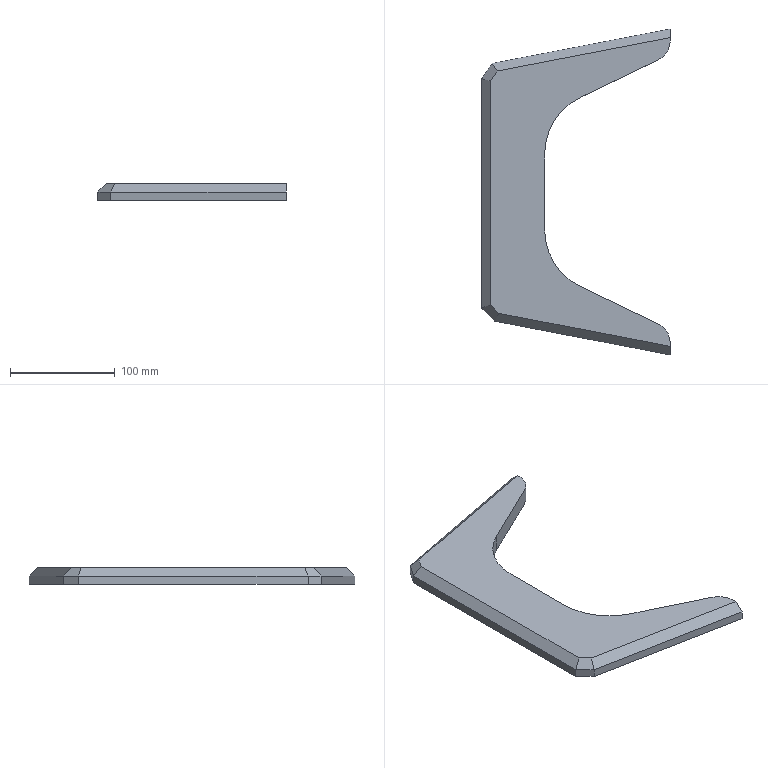Part | SolidWorks | features Chamfer 2, Extrusion 1 | 1 solid | 21 faces | box 180 x 311.6 x 16 mm | volume 387961 mm3 | plane 17 | cylinder 4 | commonest cylinder face diameters 40 x2 120 x2
STEP:
#1=CARTESIAN_POINT('',(9.818,122.898,0.));
#2=VERTEX_POINT('',#1);
#3=CARTESIAN_POINT('',(9.818,122.898,8.));
#4=VERTEX_POINT('',#3);
#5=CARTESIAN_POINT('',(9.818,122.898,16.));
#6=DIRECTION('',(0.,0.,1.));
#7=VECTOR('',#6,1000.);
#8=LINE('',#5,#7);
#9=EDGE_CURVE('',#2,#4,#8,.T.);
#10=ORIENTED_EDGE('',*,*,#9,.T.);
#11=CARTESIAN_POINT('',(180.,155.8,8.));
#12=VERTEX_POINT('',#11);
#13=CARTESIAN_POINT('',(0.,121.,8.));
#14=DIRECTION('',(0.9818,0.1898,0.));
#15=VECTOR('',#14,1000.);
#16=LINE('',#13,#15);
#17=EDGE_CURVE('',#4,#12,#16,.T.);
#18=ORIENTED_EDGE('',*,*,#17,.T.);
#19=CARTESIAN_POINT('',(180.,155.8,0.));
#20=VERTEX_POINT('',#19);
#21=CARTESIAN_POINT('',(180.,155.8,16.));
#22=DIRECTION('',(0.,0.,-1.));
#23=VECTOR('',#22,1000.);
#24=LINE('',#21,#23);
#25=EDGE_CURVE('',#12,#20,#24,.T.);
#26=ORIENTED_EDGE('',*,*,#25,.T.);
#27=CARTESIAN_POINT('',(0.,121.,0.));
#28=DIRECTION('',(-0.9818,-0.1898,0.));
#29=VECTOR('',#28,1000.);
#30=LINE('',#27,#29);
#31=EDGE_CURVE('',#20,#2,#30,.T.);
#32=ORIENTED_EDGE('',*,*,#31,.T.);
#33=EDGE_LOOP('',(#10,#18,#26,#32));
#34=FACE_OUTER_BOUND('',#33,.T.);
#35=CARTESIAN_POINT('',(0.,121.,16.));
#36=DIRECTION('',(0.1898,-0.9818,0.));
#37=DIRECTION('',(0.9818,0.1898,0.));
#38=AXIS2_PLACEMENT_3D('',#35,#36,#37);
#39=PLANE('',#38);
#40=ADVANCED_FACE('',(#34),#39,.F.);
#41=CARTESIAN_POINT('',(0.,-111.,0.));
#42=VERTEX_POINT('',#41);
#43=CARTESIAN_POINT('',(0.,-111.,8.));
#44=VERTEX_POINT('',#43);
#45=CARTESIAN_POINT('',(0.,-111.,16.));
#46=DIRECTION('',(0.,0.,1.));
#47=VECTOR('',#46,1000.);
#48=LINE('',#45,#47);
#49=EDGE_CURVE('',#42,#44,#48,.T.);
#50=ORIENTED_EDGE('',*,*,#49,.T.);
#51=CARTESIAN_POINT('',(0.,108.374,8.));
#52=VERTEX_POINT('',#51);
#53=CARTESIAN_POINT('',(0.,-121.,8.));
#54=DIRECTION('',(0.,1.,0.));
#55=VECTOR('',#54,1000.);
#56=LINE('',#53,#55);
#57=EDGE_CURVE('',#44,#52,#56,.T.);
#58=ORIENTED_EDGE('',*,*,#57,.T.);
#59=CARTESIAN_POINT('',(0.,108.374,0.));
#60=VERTEX_POINT('',#59);
#61=CARTESIAN_POINT('',(0.,108.374,16.));
#62=DIRECTION('',(0.,0.,-1.));
#63=VECTOR('',#62,1000.);
#64=LINE('',#61,#63);
#65=EDGE_CURVE('',#52,#60,#64,.T.);
#66=ORIENTED_EDGE('',*,*,#65,.T.);
#67=CARTESIAN_POINT('',(0.,-121.,0.));
#68=DIRECTION('',(0.,-1.,0.));
#69=VECTOR('',#68,1000.);
#70=LINE('',#67,#69);
#71=EDGE_CURVE('',#60,#42,#70,.T.);
#72=ORIENTED_EDGE('',*,*,#71,.T.);
#73=EDGE_LOOP('',(#50,#58,#66,#72));
#74=FACE_OUTER_BOUND('',#73,.T.);
#75=CARTESIAN_POINT('',(0.,-121.,16.));
#76=DIRECTION('',(1.,0.,0.));
#77=DIRECTION('',(0.,0.,-1.));
#78=AXIS2_PLACEMENT_3D('',#75,#76,#77);
#79=PLANE('',#78);
#80=ADVANCED_FACE('',(#74),#79,.F.);
#81=CARTESIAN_POINT('',(180.,-155.8,8.));
#82=VERTEX_POINT('',#81);
#83=CARTESIAN_POINT('',(180.,-155.8,0.));
#84=VERTEX_POINT('',#83);
#85=CARTESIAN_POINT('',(180.,-155.8,16.));
#86=DIRECTION('',(0.,0.,-1.));
#87=VECTOR('',#86,1000.);
#88=LINE('',#85,#87);
#89=EDGE_CURVE('',#82,#84,#88,.T.);
#90=ORIENTED_EDGE('',*,*,#89,.F.);
#91=CARTESIAN_POINT('',(12.397,-123.397,8.));
#92=VERTEX_POINT('',#91);
#93=CARTESIAN_POINT('',(180.,-155.8,8.));
#94=DIRECTION('',(-0.9818,0.1898,0.));
#95=VECTOR('',#94,1000.);
#96=LINE('',#93,#95);
#97=EDGE_CURVE('',#82,#92,#96,.T.);
#98=ORIENTED_EDGE('',*,*,#97,.T.);
#99=CARTESIAN_POINT('',(12.397,-123.397,0.));
#100=VERTEX_POINT('',#99);
#101=CARTESIAN_POINT('',(12.397,-123.397,16.));
#102=DIRECTION('',(0.,0.,-1.));
#103=VECTOR('',#102,1000.);
#104=LINE('',#101,#103);
#105=EDGE_CURVE('',#92,#100,#104,.T.);
#106=ORIENTED_EDGE('',*,*,#105,.T.);
#107=CARTESIAN_POINT('',(180.,-155.8,0.));
#108=DIRECTION('',(0.9818,-0.1898,0.));
#109=VECTOR('',#108,1000.);
#110=LINE('',#107,#109);
#111=EDGE_CURVE('',#100,#84,#110,.T.);
#112=ORIENTED_EDGE('',*,*,#111,.T.);
#113=EDGE_LOOP('',(#90,#98,#106,#112));
#114=FACE_OUTER_BOUND('',#113,.T.);
#115=CARTESIAN_POINT('',(180.,-155.8,16.));
#116=DIRECTION('',(0.1898,0.9818,0.));
#117=DIRECTION('',(-0.9818,0.1898,0.));
#118=AXIS2_PLACEMENT_3D('',#115,#116,#117);
#119=PLANE('',#118);
#120=ADVANCED_FACE('',(#114),#119,.F.);
#121=CARTESIAN_POINT('',(180.,-147.652,16.));
#122=VERTEX_POINT('',#121);
#123=CARTESIAN_POINT('',(180.,-144.371,16.));
#124=VERTEX_POINT('',#123);
#125=CARTESIAN_POINT('',(180.,-144.371,16.));
#126=DIRECTION('',(0.,1.,0.));
#127=VECTOR('',#126,1000.);
#128=LINE('',#125,#127);
#129=EDGE_CURVE('',#122,#124,#128,.T.);
#130=ORIENTED_EDGE('',*,*,#129,.F.);
#131=CARTESIAN_POINT('',(180.,-140.395,23.125));
#132=DIRECTION('',(0.,-0.7136,-0.7006));
#133=VECTOR('',#132,1000.);
#134=LINE('',#131,#133);
#135=EDGE_CURVE('',#122,#82,#134,.T.);
#136=ORIENTED_EDGE('',*,*,#135,.T.);
#137=ORIENTED_EDGE('',*,*,#89,.T.);
#138=CARTESIAN_POINT('',(180.,-144.371,0.));
#139=VERTEX_POINT('',#138);
#140=CARTESIAN_POINT('',(180.,-144.371,0.));
#141=DIRECTION('',(0.,1.,0.));
#142=VECTOR('',#141,1000.);
#143=LINE('',#140,#142);
#144=EDGE_CURVE('',#84,#139,#143,.T.);
#145=ORIENTED_EDGE('',*,*,#144,.T.);
#146=CARTESIAN_POINT('',(180.,-144.371,16.));
#147=DIRECTION('',(0.,0.,-1.));
#148=VECTOR('',#147,1000.);
#149=LINE('',#146,#148);
#150=EDGE_CURVE('',#124,#139,#149,.T.);
#151=ORIENTED_EDGE('',*,*,#150,.F.);
#152=EDGE_LOOP('',(#130,#136,#137,#145,#151));
#153=FACE_OUTER_BOUND('',#152,.T.);
#154=CARTESIAN_POINT('',(180.,-144.371,16.));
#155=DIRECTION('',(-1.,0.,0.));
#156=DIRECTION('',(0.,0.,1.));
#157=AXIS2_PLACEMENT_3D('',#154,#155,#156);
#158=PLANE('',#157);
#159=ADVANCED_FACE('',(#153),#158,.F.);
#160=CARTESIAN_POINT('',(168.686,-126.356,0.));
#161=VERTEX_POINT('',#160);
#162=CARTESIAN_POINT('',(160.,-144.371,0.));
#163=DIRECTION('',(0.,0.,1.));
#164=DIRECTION('',(1.,0.,0.));
#165=AXIS2_PLACEMENT_3D('',#162,#163,#164);
#166=CIRCLE('',#165,20.);
#167=EDGE_CURVE('',#139,#161,#166,.T.);
#168=ORIENTED_EDGE('',*,*,#167,.T.);
#169=CARTESIAN_POINT('',(168.686,-126.356,16.));
#170=VERTEX_POINT('',#169);
#171=CARTESIAN_POINT('',(168.686,-126.356,16.));
#172=DIRECTION('',(0.,0.,-1.));
#173=VECTOR('',#172,1000.);
#174=LINE('',#171,#173);
#175=EDGE_CURVE('',#170,#161,#174,.T.);
#176=ORIENTED_EDGE('',*,*,#175,.F.);
#177=CARTESIAN_POINT('',(160.,-144.371,16.));
#178=DIRECTION('',(0.,0.,1.));
#179=DIRECTION('',(1.,0.,0.));
#180=AXIS2_PLACEMENT_3D('',#177,#178,#179);
#181=CIRCLE('',#180,20.);
#182=EDGE_CURVE('',#124,#170,#181,.T.);
#183=ORIENTED_EDGE('',*,*,#182,.F.);
#184=ORIENTED_EDGE('',*,*,#150,.T.);
#185=EDGE_LOOP('',(#168,#176,#183,#184));
#186=FACE_OUTER_BOUND('',#185,.T.);
#187=CARTESIAN_POINT('',(160.,-144.371,16.));
#188=DIRECTION('',(0.,0.,-1.));
#189=DIRECTION('',(-1.,0.,0.));
#190=AXIS2_PLACEMENT_3D('',#187,#188,#189);
#191=CYLINDRICAL_SURFACE('',#190,20.);
#192=ADVANCED_FACE('',(#186),#191,.T.);
#193=CARTESIAN_POINT('',(93.941,-90.315,0.));
#194=VERTEX_POINT('',#193);
#195=CARTESIAN_POINT('',(93.941,-90.315,0.));
#196=DIRECTION('',(-0.9008,0.4343,0.));
#197=VECTOR('',#196,1000.);
#198=LINE('',#195,#197);
#199=EDGE_CURVE('',#161,#194,#198,.T.);
#200=ORIENTED_EDGE('',*,*,#199,.T.);
#201=CARTESIAN_POINT('',(93.941,-90.315,16.));
#202=VERTEX_POINT('',#201);
#203=CARTESIAN_POINT('',(93.941,-90.315,16.));
#204=DIRECTION('',(0.,0.,-1.));
#205=VECTOR('',#204,1000.);
#206=LINE('',#203,#205);
#207=EDGE_CURVE('',#202,#194,#206,.T.);
#208=ORIENTED_EDGE('',*,*,#207,.F.);
#209=CARTESIAN_POINT('',(93.941,-90.315,16.));
#210=DIRECTION('',(-0.9008,0.4343,0.));
#211=VECTOR('',#210,1000.);
#212=LINE('',#209,#211);
#213=EDGE_CURVE('',#170,#202,#212,.T.);
#214=ORIENTED_EDGE('',*,*,#213,.F.);
#215=ORIENTED_EDGE('',*,*,#175,.T.);
#216=EDGE_LOOP('',(#200,#208,#214,#215));
#217=FACE_OUTER_BOUND('',#216,.T.);
#218=CARTESIAN_POINT('',(93.941,-90.315,16.));
#219=DIRECTION('',(-0.4343,-0.9008,0.));
#220=DIRECTION('',(0.9008,-0.4343,0.));
#221=AXIS2_PLACEMENT_3D('',#218,#219,#220);
#222=PLANE('',#221);
#223=ADVANCED_FACE('',(#217),#222,.F.);
#224=CARTESIAN_POINT('',(60.,-36.27,0.));
#225=VERTEX_POINT('',#224);
#226=CARTESIAN_POINT('',(120.,-36.27,0.));
#227=DIRECTION('',(0.,0.,-1.));
#228=DIRECTION('',(-1.,0.,0.));
#229=AXIS2_PLACEMENT_3D('',#226,#227,#228);
#230=CIRCLE('',#229,60.);
#231=EDGE_CURVE('',#194,#225,#230,.T.);
#232=ORIENTED_EDGE('',*,*,#231,.T.);
#233=CARTESIAN_POINT('',(60.,-36.27,16.));
#234=VERTEX_POINT('',#233);
#235=CARTESIAN_POINT('',(60.,-36.27,16.));
#236=DIRECTION('',(0.,0.,-1.));
#237=VECTOR('',#236,1000.);
#238=LINE('',#235,#237);
#239=EDGE_CURVE('',#234,#225,#238,.T.);
#240=ORIENTED_EDGE('',*,*,#239,.F.);
#241=CARTESIAN_POINT('',(120.,-36.27,16.));
#242=DIRECTION('',(0.,0.,-1.));
#243=DIRECTION('',(-1.,0.,0.));
#244=AXIS2_PLACEMENT_3D('',#241,#242,#243);
#245=CIRCLE('',#244,60.);
#246=EDGE_CURVE('',#202,#234,#245,.T.);
#247=ORIENTED_EDGE('',*,*,#246,.F.);
#248=ORIENTED_EDGE('',*,*,#207,.T.);
#249=EDGE_LOOP('',(#232,#240,#247,#248));
#250=FACE_OUTER_BOUND('',#249,.T.);
#251=CARTESIAN_POINT('',(120.,-36.27,16.));
#252=DIRECTION('',(0.,0.,-1.));
#253=DIRECTION('',(-1.,0.,0.));
#254=AXIS2_PLACEMENT_3D('',#251,#252,#253);
#255=CYLINDRICAL_SURFACE('',#254,60.);
#256=ADVANCED_FACE('',(#250),#255,.F.);
#257=CARTESIAN_POINT('',(60.,36.37,0.));
#258=VERTEX_POINT('',#257);
#259=CARTESIAN_POINT('',(60.,36.37,0.));
#260=DIRECTION('',(0.,1.,0.));
#261=VECTOR('',#260,1000.);
#262=LINE('',#259,#261);
#263=EDGE_CURVE('',#225,#258,#262,.T.);
#264=ORIENTED_EDGE('',*,*,#263,.T.);
#265=CARTESIAN_POINT('',(60.,36.37,16.));
#266=VERTEX_POINT('',#265);
#267=CARTESIAN_POINT('',(60.,36.37,16.));
#268=DIRECTION('',(0.,0.,-1.));
#269=VECTOR('',#268,1000.);
#270=LINE('',#267,#269);
#271=EDGE_CURVE('',#266,#258,#270,.T.);
#272=ORIENTED_EDGE('',*,*,#271,.F.);
#273=CARTESIAN_POINT('',(60.,36.37,16.));
#274=DIRECTION('',(0.,1.,0.));
#275=VECTOR('',#274,1000.);
#276=LINE('',#273,#275);
#277=EDGE_CURVE('',#234,#266,#276,.T.);
#278=ORIENTED_EDGE('',*,*,#277,.F.);
#279=ORIENTED_EDGE('',*,*,#239,.T.);
#280=EDGE_LOOP('',(#264,#272,#278,#279));
#281=FACE_OUTER_BOUND('',#280,.T.);
#282=CARTESIAN_POINT('',(60.,36.37,16.));
#283=DIRECTION('',(-1.,0.,0.));
#284=DIRECTION('',(0.,-1.,0.));
#285=AXIS2_PLACEMENT_3D('',#282,#283,#284);
#286=PLANE('',#285);
#287=ADVANCED_FACE('',(#281),#286,.F.);
#288=CARTESIAN_POINT('',(93.941,90.415,0.));
#289=VERTEX_POINT('',#288);
#290=CARTESIAN_POINT('',(120.,36.37,0.));
#291=DIRECTION('',(0.,0.,-1.));
#292=DIRECTION('',(-1.,0.,0.));
#293=AXIS2_PLACEMENT_3D('',#290,#291,#292);
#294=CIRCLE('',#293,60.);
#295=EDGE_CURVE('',#258,#289,#294,.T.);
#296=ORIENTED_EDGE('',*,*,#295,.T.);
#297=CARTESIAN_POINT('',(93.941,90.415,16.));
#298=VERTEX_POINT('',#297);
#299=CARTESIAN_POINT('',(93.941,90.415,16.));
#300=DIRECTION('',(0.,0.,-1.));
#301=VECTOR('',#300,1000.);
#302=LINE('',#299,#301);
#303=EDGE_CURVE('',#298,#289,#302,.T.);
#304=ORIENTED_EDGE('',*,*,#303,.F.);
#305=CARTESIAN_POINT('',(120.,36.37,16.));
#306=DIRECTION('',(0.,0.,-1.));
#307=DIRECTION('',(-1.,0.,0.));
#308=AXIS2_PLACEMENT_3D('',#305,#306,#307);
#309=CIRCLE('',#308,60.);
#310=EDGE_CURVE('',#266,#298,#309,.T.);
#311=ORIENTED_EDGE('',*,*,#310,.F.);
#312=ORIENTED_EDGE('',*,*,#271,.T.);
#313=EDGE_LOOP('',(#296,#304,#311,#312));
#314=FACE_OUTER_BOUND('',#313,.T.);
#315=CARTESIAN_POINT('',(120.,36.37,16.));
#316=DIRECTION('',(0.,0.,-1.));
#317=DIRECTION('',(-1.,0.,0.));
#318=AXIS2_PLACEMENT_3D('',#315,#316,#317);
#319=CYLINDRICAL_SURFACE('',#318,60.);
#320=ADVANCED_FACE('',(#314),#319,.F.);
#321=CARTESIAN_POINT('',(168.686,126.456,0.));
#322=VERTEX_POINT('',#321);
#323=CARTESIAN_POINT('',(168.686,126.456,0.));
#324=DIRECTION('',(0.9008,0.4343,0.));
#325=VECTOR('',#324,1000.);
#326=LINE('',#323,#325);
#327=EDGE_CURVE('',#289,#322,#326,.T.);
#328=ORIENTED_EDGE('',*,*,#327,.T.);
#329=CARTESIAN_POINT('',(168.686,126.456,16.));
#330=VERTEX_POINT('',#329);
#331=CARTESIAN_POINT('',(168.686,126.456,16.));
#332=DIRECTION('',(0.,0.,-1.));
#333=VECTOR('',#332,1000.);
#334=LINE('',#331,#333);
#335=EDGE_CURVE('',#330,#322,#334,.T.);
#336=ORIENTED_EDGE('',*,*,#335,.F.);
#337=CARTESIAN_POINT('',(168.686,126.456,16.));
#338=DIRECTION('',(0.9008,0.4343,0.));
#339=VECTOR('',#338,1000.);
#340=LINE('',#337,#339);
#341=EDGE_CURVE('',#298,#330,#340,.T.);
#342=ORIENTED_EDGE('',*,*,#341,.F.);
#343=ORIENTED_EDGE('',*,*,#303,.T.);
#344=EDGE_LOOP('',(#328,#336,#342,#343));
#345=FACE_OUTER_BOUND('',#344,.T.);
#346=CARTESIAN_POINT('',(168.686,126.456,16.));
#347=DIRECTION('',(-0.4343,0.9008,0.));
#348=DIRECTION('',(-0.9008,-0.4343,0.));
#349=AXIS2_PLACEMENT_3D('',#346,#347,#348);
#350=PLANE('',#349);
#351=ADVANCED_FACE('',(#345),#350,.F.);
#352=CARTESIAN_POINT('',(180.,144.471,0.));
#353=VERTEX_POINT('',#352);
#354=CARTESIAN_POINT('',(160.,144.471,0.));
#355=DIRECTION('',(0.,0.,1.));
#356=DIRECTION('',(-1.,0.,0.));
#357=AXIS2_PLACEMENT_3D('',#354,#355,#356);
#358=CIRCLE('',#357,20.);
#359=EDGE_CURVE('',#322,#353,#358,.T.);
#360=ORIENTED_EDGE('',*,*,#359,.T.);
#361=CARTESIAN_POINT('',(180.,144.471,16.));
#362=VERTEX_POINT('',#361);
#363=CARTESIAN_POINT('',(180.,144.471,16.));
#364=DIRECTION('',(0.,0.,-1.));
#365=VECTOR('',#364,1000.);
#366=LINE('',#363,#365);
#367=EDGE_CURVE('',#362,#353,#366,.T.);
#368=ORIENTED_EDGE('',*,*,#367,.F.);
#369=CARTESIAN_POINT('',(160.,144.471,16.));
#370=DIRECTION('',(0.,0.,1.));
#371=DIRECTION('',(-1.,0.,0.));
#372=AXIS2_PLACEMENT_3D('',#369,#370,#371);
#373=CIRCLE('',#372,20.);
#374=EDGE_CURVE('',#330,#362,#373,.T.);
#375=ORIENTED_EDGE('',*,*,#374,.F.);
#376=ORIENTED_EDGE('',*,*,#335,.T.);
#377=EDGE_LOOP('',(#360,#368,#375,#376));
#378=FACE_OUTER_BOUND('',#377,.T.);
#379=CARTESIAN_POINT('',(160.,144.471,16.));
#380=DIRECTION('',(0.,0.,-1.));
#381=DIRECTION('',(-1.,0.,0.));
#382=AXIS2_PLACEMENT_3D('',#379,#380,#381);
#383=CYLINDRICAL_SURFACE('',#382,20.);
#384=ADVANCED_FACE('',(#378),#383,.T.);
#385=ORIENTED_EDGE('',*,*,#25,.F.);
#386=CARTESIAN_POINT('',(180.,147.652,16.));
#387=VERTEX_POINT('',#386);
#388=CARTESIAN_POINT('',(180.,145.696,17.921));
#389=DIRECTION('',(0.,-0.7136,0.7006));
#390=VECTOR('',#389,1000.);
#391=LINE('',#388,#390);
#392=EDGE_CURVE('',#12,#387,#391,.T.);
#393=ORIENTED_EDGE('',*,*,#392,.T.);
#394=CARTESIAN_POINT('',(180.,155.8,16.));
#395=DIRECTION('',(0.,1.,0.));
#396=VECTOR('',#395,1000.);
#397=LINE('',#394,#396);
#398=EDGE_CURVE('',#362,#387,#397,.T.);
#399=ORIENTED_EDGE('',*,*,#398,.F.);
#400=ORIENTED_EDGE('',*,*,#367,.T.);
#401=CARTESIAN_POINT('',(180.,155.8,0.));
#402=DIRECTION('',(0.,1.,0.));
#403=VECTOR('',#402,1000.);
#404=LINE('',#401,#403);
#405=EDGE_CURVE('',#353,#20,#404,.T.);
#406=ORIENTED_EDGE('',*,*,#405,.T.);
#407=EDGE_LOOP('',(#385,#393,#399,#400,#406));
#408=FACE_OUTER_BOUND('',#407,.T.);
#409=CARTESIAN_POINT('',(180.,155.8,16.));
#410=DIRECTION('',(-1.,0.,0.));
#411=DIRECTION('',(0.,0.,1.));
#412=AXIS2_PLACEMENT_3D('',#409,#410,#411);
#413=PLANE('',#412);
#414=ADVANCED_FACE('',(#408),#413,.F.);
#415=ORIENTED_EDGE('',*,*,#398,.T.);
#416=CARTESIAN_POINT('',(14.59,115.673,16.));
#417=VERTEX_POINT('',#416);
#418=CARTESIAN_POINT('',(160.128,143.81,16.));
#419=DIRECTION('',(-0.9818,-0.1898,0.));
#420=VECTOR('',#419,1000.);
#421=LINE('',#418,#420);
#422=EDGE_CURVE('',#387,#417,#421,.T.);
#423=ORIENTED_EDGE('',*,*,#422,.T.);
#424=CARTESIAN_POINT('',(8.,105.923,16.));
#425=VERTEX_POINT('',#424);
#426=CARTESIAN_POINT('',(6.628,103.894,16.));
#427=DIRECTION('',(-0.56,-0.8285,0.));
#428=VECTOR('',#427,1000.);
#429=LINE('',#426,#428);
#430=EDGE_CURVE('',#417,#425,#429,.T.);
#431=ORIENTED_EDGE('',*,*,#430,.T.);
#432=CARTESIAN_POINT('',(8.,-107.686,16.));
#433=VERTEX_POINT('',#432);
#434=CARTESIAN_POINT('',(8.,144.471,16.));
#435=DIRECTION('',(0.,-1.,0.));
#436=VECTOR('',#435,1000.);
#437=LINE('',#434,#436);
#438=EDGE_CURVE('',#425,#433,#437,.T.);
#439=ORIENTED_EDGE('',*,*,#438,.T.);
#440=CARTESIAN_POINT('',(16.321,-116.007,16.));
#441=VERTEX_POINT('',#440);
#442=CARTESIAN_POINT('',(18.054,-117.74,16.));
#443=DIRECTION('',(0.7071,-0.7071,0.));
#444=VECTOR('',#443,1000.);
#445=LINE('',#442,#444);
#446=EDGE_CURVE('',#433,#441,#445,.T.);
#447=ORIENTED_EDGE('',*,*,#446,.T.);
#448=CARTESIAN_POINT('',(106.278,-133.399,16.));
#449=DIRECTION('',(0.9818,-0.1898,0.));
#450=VECTOR('',#449,1000.);
#451=LINE('',#448,#450);
#452=EDGE_CURVE('',#441,#122,#451,.T.);
#453=ORIENTED_EDGE('',*,*,#452,.T.);
#454=ORIENTED_EDGE('',*,*,#129,.T.);
#455=ORIENTED_EDGE('',*,*,#182,.T.);
#456=ORIENTED_EDGE('',*,*,#213,.T.);
#457=ORIENTED_EDGE('',*,*,#246,.T.);
#458=ORIENTED_EDGE('',*,*,#277,.T.);
#459=ORIENTED_EDGE('',*,*,#310,.T.);
#460=ORIENTED_EDGE('',*,*,#341,.T.);
#461=ORIENTED_EDGE('',*,*,#374,.T.);
#462=EDGE_LOOP('',(#415,#423,#431,#439,#447,#453,#454,#455,#456,#457,#458,#459,#460,#461));
#463=FACE_OUTER_BOUND('',#462,.T.);
#464=CARTESIAN_POINT('',(160.,144.471,16.));
#465=DIRECTION('',(0.,0.,-1.));
#466=DIRECTION('',(-1.,0.,0.));
#467=AXIS2_PLACEMENT_3D('',#464,#465,#466);
#468=PLANE('',#467);
#469=ADVANCED_FACE('',(#463),#468,.F.);
#470=ORIENTED_EDGE('',*,*,#71,.F.);
#471=CARTESIAN_POINT('',(66.929,207.385,0.));
#472=DIRECTION('',(0.56,0.8285,0.));
#473=VECTOR('',#472,1000.);
#474=LINE('',#471,#473);
#475=EDGE_CURVE('',#60,#2,#474,.T.);
#476=ORIENTED_EDGE('',*,*,#475,.T.);
#477=ORIENTED_EDGE('',*,*,#31,.F.);
#478=ORIENTED_EDGE('',*,*,#405,.F.);
#479=ORIENTED_EDGE('',*,*,#359,.F.);
#480=ORIENTED_EDGE('',*,*,#327,.F.);
#481=ORIENTED_EDGE('',*,*,#295,.F.);
#482=ORIENTED_EDGE('',*,*,#263,.F.);
#483=ORIENTED_EDGE('',*,*,#231,.F.);
#484=ORIENTED_EDGE('',*,*,#199,.F.);
#485=ORIENTED_EDGE('',*,*,#167,.F.);
#486=ORIENTED_EDGE('',*,*,#144,.F.);
#487=ORIENTED_EDGE('',*,*,#111,.F.);
#488=CARTESIAN_POINT('',(-47.735,-63.265,0.));
#489=DIRECTION('',(-0.7071,0.7071,0.));
#490=VECTOR('',#489,1000.);
#491=LINE('',#488,#490);
#492=EDGE_CURVE('',#100,#42,#491,.T.);
#493=ORIENTED_EDGE('',*,*,#492,.T.);
#494=EDGE_LOOP('',(#470,#476,#477,#478,#479,#480,#481,#482,#483,#484,#485,#486,#487,#493));
#495=FACE_OUTER_BOUND('',#494,.T.);
#496=CARTESIAN_POINT('',(160.,144.471,0.));
#497=DIRECTION('',(0.,0.,-1.));
#498=DIRECTION('',(-1.,0.,0.));
#499=AXIS2_PLACEMENT_3D('',#496,#497,#498);
#500=PLANE('',#499);
#501=ADVANCED_FACE('',(#495),#500,.T.);
#502=ORIENTED_EDGE('',*,*,#65,.F.);
#503=CARTESIAN_POINT('',(9.818,122.898,8.));
#504=DIRECTION('',(0.56,0.8285,0.));
#505=VECTOR('',#504,1000.);
#506=LINE('',#503,#505);
#507=EDGE_CURVE('',#52,#4,#506,.T.);
#508=ORIENTED_EDGE('',*,*,#507,.T.);
#509=ORIENTED_EDGE('',*,*,#9,.F.);
#510=ORIENTED_EDGE('',*,*,#475,.F.);
#511=EDGE_LOOP('',(#502,#508,#509,#510));
#512=FACE_OUTER_BOUND('',#511,.T.);
#513=CARTESIAN_POINT('',(0.,108.374,16.));
#514=DIRECTION('',(0.8285,-0.56,0.));
#515=DIRECTION('',(0.56,0.8285,0.));
#516=AXIS2_PLACEMENT_3D('',#513,#514,#515);
#517=PLANE('',#516);
#518=ADVANCED_FACE('',(#512),#517,.F.);
#519=ORIENTED_EDGE('',*,*,#105,.F.);
#520=CARTESIAN_POINT('',(0.,-111.,8.));
#521=DIRECTION('',(-0.7071,0.7071,0.));
#522=VECTOR('',#521,1000.);
#523=LINE('',#520,#522);
#524=EDGE_CURVE('',#92,#44,#523,.T.);
#525=ORIENTED_EDGE('',*,*,#524,.T.);
#526=ORIENTED_EDGE('',*,*,#49,.F.);
#527=ORIENTED_EDGE('',*,*,#492,.F.);
#528=EDGE_LOOP('',(#519,#525,#526,#527));
#529=FACE_OUTER_BOUND('',#528,.T.);
#530=CARTESIAN_POINT('',(12.397,-123.397,16.));
#531=DIRECTION('',(0.7071,0.7071,0.));
#532=DIRECTION('',(-0.7071,0.7071,0.));
#533=AXIS2_PLACEMENT_3D('',#530,#531,#532);
#534=PLANE('',#533);
#535=ADVANCED_FACE('',(#529),#534,.F.);
#536=ORIENTED_EDGE('',*,*,#135,.F.);
#537=ORIENTED_EDGE('',*,*,#452,.F.);
#538=CARTESIAN_POINT('',(22.895,-103.627,29.403));
#539=DIRECTION('',(0.339,0.6383,0.6911));
#540=VECTOR('',#539,1000.);
#541=LINE('',#538,#540);
#542=EDGE_CURVE('',#92,#441,#541,.T.);
#543=ORIENTED_EDGE('',*,*,#542,.F.);
#544=ORIENTED_EDGE('',*,*,#97,.F.);
#545=EDGE_LOOP('',(#536,#537,#543,#544));
#546=FACE_OUTER_BOUND('',#545,.T.);
#547=CARTESIAN_POINT('',(106.278,-133.399,16.));
#548=DIRECTION('',(0.1342,0.6943,-0.7071));
#549=DIRECTION('',(0.,0.7136,0.7006));
#550=AXIS2_PLACEMENT_3D('',#547,#548,#549);
#551=PLANE('',#550);
#552=ADVANCED_FACE('',(#546),#551,.F.);
#553=ORIENTED_EDGE('',*,*,#542,.T.);
#554=ORIENTED_EDGE('',*,*,#446,.F.);
#555=CARTESIAN_POINT('',(-5.509,-113.282,2.491));
#556=DIRECTION('',(0.6786,0.2811,0.6786));
#557=VECTOR('',#556,1000.);
#558=LINE('',#555,#557);
#559=EDGE_CURVE('',#44,#433,#558,.T.);
#560=ORIENTED_EDGE('',*,*,#559,.F.);
#561=ORIENTED_EDGE('',*,*,#524,.F.);
#562=EDGE_LOOP('',(#553,#554,#560,#561));
#563=FACE_OUTER_BOUND('',#562,.T.);
#564=CARTESIAN_POINT('',(-42.079,-57.608,16.));
#565=DIRECTION('',(0.5,0.5,-0.7071));
#566=DIRECTION('',(-0.8165,0.,-0.5774));
#567=AXIS2_PLACEMENT_3D('',#564,#565,#566);
#568=PLANE('',#567);
#569=ADVANCED_FACE('',(#563),#568,.F.);
#570=ORIENTED_EDGE('',*,*,#559,.T.);
#571=ORIENTED_EDGE('',*,*,#438,.F.);
#572=CARTESIAN_POINT('',(2.361,107.651,10.361));
#573=DIRECTION('',(0.6911,-0.2117,0.6911));
#574=VECTOR('',#573,1000.);
#575=LINE('',#572,#574);
#576=EDGE_CURVE('',#52,#425,#575,.T.);
#577=ORIENTED_EDGE('',*,*,#576,.F.);
#578=ORIENTED_EDGE('',*,*,#57,.F.);
#579=EDGE_LOOP('',(#570,#571,#577,#578));
#580=FACE_OUTER_BOUND('',#579,.T.);
#581=CARTESIAN_POINT('',(8.,144.471,16.));
#582=DIRECTION('',(0.7071,0.,-0.7071));
#583=DIRECTION('',(-0.7071,0.,-0.7071));
#584=AXIS2_PLACEMENT_3D('',#581,#582,#583);
#585=PLANE('',#584);
#586=ADVANCED_FACE('',(#580),#585,.F.);
#587=ORIENTED_EDGE('',*,*,#576,.T.);
#588=ORIENTED_EDGE('',*,*,#430,.F.);
#589=CARTESIAN_POINT('',(2.61,133.812,-4.084));
#590=DIRECTION('',(0.4048,-0.6129,0.6786));
#591=VECTOR('',#590,1000.);
#592=LINE('',#589,#591);
#593=EDGE_CURVE('',#4,#417,#592,.T.);
#594=ORIENTED_EDGE('',*,*,#593,.F.);
#595=ORIENTED_EDGE('',*,*,#507,.F.);
#596=EDGE_LOOP('',(#587,#588,#594,#595));
#597=FACE_OUTER_BOUND('',#596,.T.);
#598=CARTESIAN_POINT('',(73.557,202.905,16.));
#599=DIRECTION('',(0.5858,-0.396,-0.7071));
#600=DIRECTION('',(-0.7701,0.,-0.638));
#601=AXIS2_PLACEMENT_3D('',#598,#599,#600);
#602=PLANE('',#601);
#603=ADVANCED_FACE('',(#597),#602,.F.);
#604=ORIENTED_EDGE('',*,*,#392,.F.);
#605=ORIENTED_EDGE('',*,*,#17,.F.);
#606=ORIENTED_EDGE('',*,*,#593,.T.);
#607=ORIENTED_EDGE('',*,*,#422,.F.);
#608=EDGE_LOOP('',(#604,#605,#606,#607));
#609=FACE_OUTER_BOUND('',#608,.T.);
#610=CARTESIAN_POINT('',(160.128,143.81,16.));
#611=DIRECTION('',(0.1342,-0.6943,-0.7071));
#612=DIRECTION('',(0.,0.7136,-0.7006));
#613=AXIS2_PLACEMENT_3D('',#610,#611,#612);
#614=PLANE('',#613);
#615=ADVANCED_FACE('',(#609),#614,.F.);
#616=CLOSED_SHELL('',(#40,#80,#120,#159,#192,#223,#256,#287,#320,#351,#384,#414,#469,#501,#518,#535,#552,#569,#586,#603,#615));
#617=MANIFOLD_SOLID_BREP('',#616);
#618=CARTESIAN_POINT('',(0.,0.,0.));
#619=DIRECTION('',(0.,0.,1.));
#620=DIRECTION('',(1.,0.,0.));
#621=AXIS2_PLACEMENT_3D('',#618,#619,#620);
#622=(LENGTH_UNIT()NAMED_UNIT(*)SI_UNIT(.MILLI.,.METRE.));
#623=UNCERTAINTY_MEASURE_WITH_UNIT(LENGTH_MEASURE(0.00001),#622,'','');
#624=(NAMED_UNIT(*)PLANE_ANGLE_UNIT()SI_UNIT($,.RADIAN.));
#625=(NAMED_UNIT(*)SI_UNIT($,.STERADIAN.)SOLID_ANGLE_UNIT());
#626=(GEOMETRIC_REPRESENTATION_CONTEXT(3)GLOBAL_UNCERTAINTY_ASSIGNED_CONTEXT((#623))GLOBAL_UNIT_ASSIGNED_CONTEXT((#622,#624,#625))REPRESENTATION_CONTEXT('',''));
#627=ADVANCED_BREP_SHAPE_REPRESENTATION('',(#617,#621),#626);